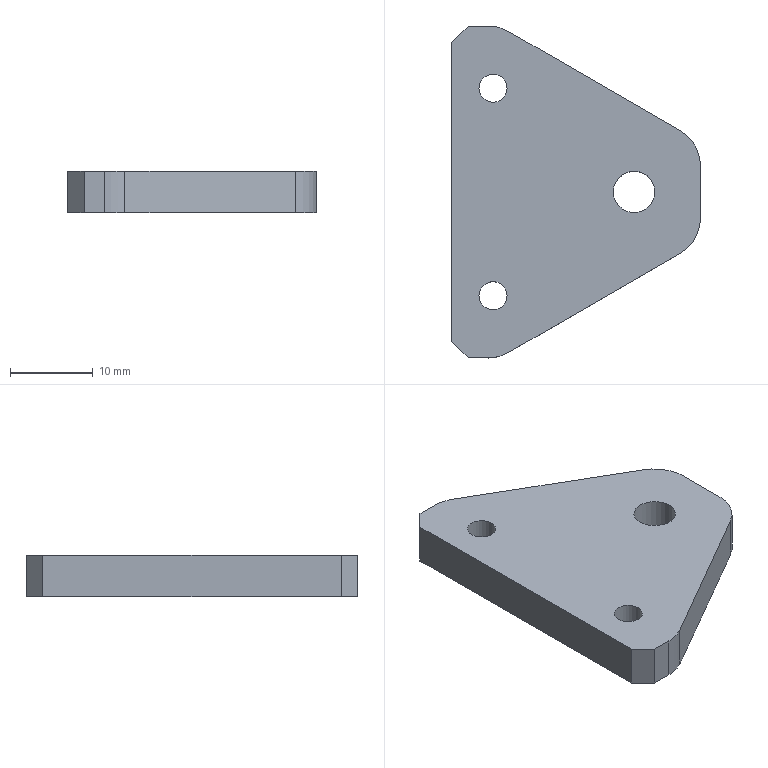Part | NX | 1 solid | 17 faces | box 30 x 40 x 5 mm | volume 4079 mm3 | plane 10 | cylinder 7 | commonest cylinder face diameters 10 x4 3.4 x2 5 x1
STEP:
#1=CARTESIAN_POINT('',(15.,-3.113,0.));
#2=VERTEX_POINT('',#1);
#3=CARTESIAN_POINT('',(15.,3.113,0.));
#4=VERTEX_POINT('',#3);
#5=CARTESIAN_POINT('',(15.,-20.,0.));
#6=DIRECTION('',(0.,1.,0.));
#7=VECTOR('',#6,1000.);
#8=LINE('',#5,#7);
#9=EDGE_CURVE('',#2,#4,#8,.T.);
#10=ORIENTED_EDGE('',*,*,#9,.F.);
#11=CARTESIAN_POINT('',(15.,-3.113,-5.));
#12=VERTEX_POINT('',#11);
#13=CARTESIAN_POINT('',(15.,-3.113,-5.));
#14=DIRECTION('',(0.,0.,1.));
#15=VECTOR('',#14,1000.);
#16=LINE('',#13,#15);
#17=EDGE_CURVE('',#2,#12,#16,.F.);
#18=ORIENTED_EDGE('',*,*,#17,.T.);
#19=CARTESIAN_POINT('',(15.,3.113,-5.));
#20=VERTEX_POINT('',#19);
#21=CARTESIAN_POINT('',(15.,-20.,-5.));
#22=DIRECTION('',(0.,1.,0.));
#23=VECTOR('',#22,1000.);
#24=LINE('',#21,#23);
#25=EDGE_CURVE('',#12,#20,#24,.T.);
#26=ORIENTED_EDGE('',*,*,#25,.T.);
#27=CARTESIAN_POINT('',(15.,3.113,-5.));
#28=DIRECTION('',(0.,0.,-1.));
#29=VECTOR('',#28,1000.);
#30=LINE('',#27,#29);
#31=EDGE_CURVE('',#20,#4,#30,.F.);
#32=ORIENTED_EDGE('',*,*,#31,.T.);
#33=EDGE_LOOP('',(#10,#18,#26,#32));
#34=FACE_BOUND('',#33,.T.);
#35=CARTESIAN_POINT('',(15.,-20.,-5.));
#36=DIRECTION('',(1.,0.,0.));
#37=DIRECTION('',(0.,0.,-1.));
#38=AXIS2_PLACEMENT_3D('',#35,#36,#37);
#39=PLANE('',#38);
#40=ADVANCED_FACE('',(#34),#39,.T.);
#41=CARTESIAN_POINT('',(-8.3,12.5,-5.));
#42=VERTEX_POINT('',#41);
#43=CARTESIAN_POINT('',(-10.,12.5,-5.));
#44=DIRECTION('',(0.,0.,1.));
#45=DIRECTION('',(1.,0.,0.));
#46=AXIS2_PLACEMENT_3D('',#43,#44,#45);
#47=CIRCLE('',#46,1.7);
#48=EDGE_CURVE('',#42,#42,#47,.T.);
#49=ORIENTED_EDGE('',*,*,#48,.T.);
#50=EDGE_LOOP('',(#49));
#51=FACE_BOUND('',#50,.T.);
#52=CARTESIAN_POINT('',(-8.3,-12.5,-5.));
#53=VERTEX_POINT('',#52);
#54=CARTESIAN_POINT('',(-10.,-12.5,-5.));
#55=DIRECTION('',(0.,0.,1.));
#56=DIRECTION('',(1.,0.,0.));
#57=AXIS2_PLACEMENT_3D('',#54,#55,#56);
#58=CIRCLE('',#57,1.7);
#59=EDGE_CURVE('',#53,#53,#58,.T.);
#60=ORIENTED_EDGE('',*,*,#59,.T.);
#61=EDGE_LOOP('',(#60));
#62=FACE_BOUND('',#61,.T.);
#63=CARTESIAN_POINT('',(9.5,0.,-5.));
#64=VERTEX_POINT('',#63);
#65=CARTESIAN_POINT('',(7.,0.,-5.));
#66=DIRECTION('',(0.,0.,1.));
#67=DIRECTION('',(1.,0.,0.));
#68=AXIS2_PLACEMENT_3D('',#65,#66,#67);
#69=CIRCLE('',#68,2.5);
#70=EDGE_CURVE('',#64,#64,#69,.T.);
#71=ORIENTED_EDGE('',*,*,#70,.T.);
#72=EDGE_LOOP('',(#71));
#73=FACE_BOUND('',#72,.T.);
#74=CARTESIAN_POINT('',(-13.,-20.,-5.));
#75=VERTEX_POINT('',#74);
#76=CARTESIAN_POINT('',(-10.588,-20.,-5.));
#77=VERTEX_POINT('',#76);
#78=CARTESIAN_POINT('',(-15.,-20.,-5.));
#79=DIRECTION('',(1.,0.,0.));
#80=VECTOR('',#79,1000.);
#81=LINE('',#78,#80);
#82=EDGE_CURVE('',#75,#77,#81,.T.);
#83=ORIENTED_EDGE('',*,*,#82,.F.);
#84=CARTESIAN_POINT('',(-15.,-18.,-5.));
#85=VERTEX_POINT('',#84);
#86=CARTESIAN_POINT('',(-16.5,-16.5,-5.));
#87=DIRECTION('',(0.7071,-0.7071,0.));
#88=VECTOR('',#87,1000.);
#89=LINE('',#86,#88);
#90=EDGE_CURVE('',#75,#85,#89,.F.);
#91=ORIENTED_EDGE('',*,*,#90,.T.);
#92=CARTESIAN_POINT('',(-15.,18.,-5.));
#93=VERTEX_POINT('',#92);
#94=CARTESIAN_POINT('',(-15.,-20.,-5.));
#95=DIRECTION('',(0.,-1.,0.));
#96=VECTOR('',#95,1000.);
#97=LINE('',#94,#96);
#98=EDGE_CURVE('',#93,#85,#97,.T.);
#99=ORIENTED_EDGE('',*,*,#98,.F.);
#100=CARTESIAN_POINT('',(-13.,20.,-5.));
#101=VERTEX_POINT('',#100);
#102=CARTESIAN_POINT('',(-16.5,16.5,-5.));
#103=DIRECTION('',(-0.7071,-0.7071,0.));
#104=VECTOR('',#103,1000.);
#105=LINE('',#102,#104);
#106=EDGE_CURVE('',#93,#101,#105,.F.);
#107=ORIENTED_EDGE('',*,*,#106,.T.);
#108=CARTESIAN_POINT('',(-10.588,20.,-5.));
#109=VERTEX_POINT('',#108);
#110=CARTESIAN_POINT('',(-15.,20.,-5.));
#111=DIRECTION('',(-1.,0.,0.));
#112=VECTOR('',#111,1000.);
#113=LINE('',#110,#112);
#114=EDGE_CURVE('',#109,#101,#113,.T.);
#115=ORIENTED_EDGE('',*,*,#114,.F.);
#116=CARTESIAN_POINT('',(-8.088,19.33,-5.));
#117=VERTEX_POINT('',#116);
#118=CARTESIAN_POINT('',(-10.588,15.,-5.));
#119=DIRECTION('',(0.,0.,-1.));
#120=DIRECTION('',(-1.,0.,0.));
#121=AXIS2_PLACEMENT_3D('',#118,#119,#120);
#122=CIRCLE('',#121,5.);
#123=EDGE_CURVE('',#109,#117,#122,.T.);
#124=ORIENTED_EDGE('',*,*,#123,.T.);
#125=CARTESIAN_POINT('',(12.5,7.443,-5.));
#126=VERTEX_POINT('',#125);
#127=CARTESIAN_POINT('',(-9.249,20.,-5.));
#128=DIRECTION('',(0.866,-0.5,0.));
#129=VECTOR('',#128,1000.);
#130=LINE('',#127,#129);
#131=EDGE_CURVE('',#117,#126,#130,.T.);
#132=ORIENTED_EDGE('',*,*,#131,.T.);
#133=CARTESIAN_POINT('',(10.,3.113,-5.));
#134=DIRECTION('',(0.,0.,-1.));
#135=DIRECTION('',(-1.,0.,0.));
#136=AXIS2_PLACEMENT_3D('',#133,#134,#135);
#137=CIRCLE('',#136,5.);
#138=EDGE_CURVE('',#126,#20,#137,.T.);
#139=ORIENTED_EDGE('',*,*,#138,.T.);
#140=ORIENTED_EDGE('',*,*,#25,.F.);
#141=CARTESIAN_POINT('',(12.5,-7.443,-5.));
#142=VERTEX_POINT('',#141);
#143=CARTESIAN_POINT('',(10.,-3.113,-5.));
#144=DIRECTION('',(0.,0.,-1.));
#145=DIRECTION('',(-1.,0.,0.));
#146=AXIS2_PLACEMENT_3D('',#143,#144,#145);
#147=CIRCLE('',#146,5.);
#148=EDGE_CURVE('',#12,#142,#147,.T.);
#149=ORIENTED_EDGE('',*,*,#148,.T.);
#150=CARTESIAN_POINT('',(-8.088,-19.33,-5.));
#151=VERTEX_POINT('',#150);
#152=CARTESIAN_POINT('',(-9.249,-20.,-5.));
#153=DIRECTION('',(0.866,0.5,0.));
#154=VECTOR('',#153,1000.);
#155=LINE('',#152,#154);
#156=EDGE_CURVE('',#151,#142,#155,.T.);
#157=ORIENTED_EDGE('',*,*,#156,.F.);
#158=CARTESIAN_POINT('',(-10.588,-15.,-5.));
#159=DIRECTION('',(0.,0.,-1.));
#160=DIRECTION('',(-1.,0.,0.));
#161=AXIS2_PLACEMENT_3D('',#158,#159,#160);
#162=CIRCLE('',#161,5.);
#163=EDGE_CURVE('',#151,#77,#162,.T.);
#164=ORIENTED_EDGE('',*,*,#163,.T.);
#165=EDGE_LOOP('',(#83,#91,#99,#107,#115,#124,#132,#139,#140,#149,#157,#164));
#166=FACE_BOUND('',#165,.T.);
#167=CARTESIAN_POINT('',(0.,0.,-5.));
#168=DIRECTION('',(0.,0.,-1.));
#169=DIRECTION('',(-1.,0.,0.));
#170=AXIS2_PLACEMENT_3D('',#167,#168,#169);
#171=PLANE('',#170);
#172=ADVANCED_FACE('',(#51,#62,#73,#166),#171,.T.);
#173=CARTESIAN_POINT('',(-8.3,12.5,0.));
#174=VERTEX_POINT('',#173);
#175=CARTESIAN_POINT('',(-10.,12.5,0.));
#176=DIRECTION('',(0.,0.,1.));
#177=DIRECTION('',(1.,0.,0.));
#178=AXIS2_PLACEMENT_3D('',#175,#176,#177);
#179=CIRCLE('',#178,1.7);
#180=EDGE_CURVE('',#174,#174,#179,.T.);
#181=ORIENTED_EDGE('',*,*,#180,.F.);
#182=EDGE_LOOP('',(#181));
#183=FACE_BOUND('',#182,.T.);
#184=CARTESIAN_POINT('',(-8.3,-12.5,0.));
#185=VERTEX_POINT('',#184);
#186=CARTESIAN_POINT('',(-10.,-12.5,0.));
#187=DIRECTION('',(0.,0.,1.));
#188=DIRECTION('',(1.,0.,0.));
#189=AXIS2_PLACEMENT_3D('',#186,#187,#188);
#190=CIRCLE('',#189,1.7);
#191=EDGE_CURVE('',#185,#185,#190,.T.);
#192=ORIENTED_EDGE('',*,*,#191,.F.);
#193=EDGE_LOOP('',(#192));
#194=FACE_BOUND('',#193,.T.);
#195=CARTESIAN_POINT('',(9.5,0.,0.));
#196=VERTEX_POINT('',#195);
#197=CARTESIAN_POINT('',(7.,0.,0.));
#198=DIRECTION('',(0.,0.,1.));
#199=DIRECTION('',(1.,0.,0.));
#200=AXIS2_PLACEMENT_3D('',#197,#198,#199);
#201=CIRCLE('',#200,2.5);
#202=EDGE_CURVE('',#196,#196,#201,.T.);
#203=ORIENTED_EDGE('',*,*,#202,.F.);
#204=EDGE_LOOP('',(#203));
#205=FACE_BOUND('',#204,.T.);
#206=CARTESIAN_POINT('',(-15.,18.,0.));
#207=VERTEX_POINT('',#206);
#208=CARTESIAN_POINT('',(-15.,-18.,0.));
#209=VERTEX_POINT('',#208);
#210=CARTESIAN_POINT('',(-15.,-20.,0.));
#211=DIRECTION('',(0.,-1.,0.));
#212=VECTOR('',#211,1000.);
#213=LINE('',#210,#212);
#214=EDGE_CURVE('',#207,#209,#213,.T.);
#215=ORIENTED_EDGE('',*,*,#214,.T.);
#216=CARTESIAN_POINT('',(-13.,-20.,0.));
#217=VERTEX_POINT('',#216);
#218=CARTESIAN_POINT('',(-15.,-18.,0.));
#219=DIRECTION('',(-0.7071,0.7071,0.));
#220=VECTOR('',#219,1000.);
#221=LINE('',#218,#220);
#222=EDGE_CURVE('',#209,#217,#221,.F.);
#223=ORIENTED_EDGE('',*,*,#222,.T.);
#224=CARTESIAN_POINT('',(-10.588,-20.,0.));
#225=VERTEX_POINT('',#224);
#226=CARTESIAN_POINT('',(-15.,-20.,0.));
#227=DIRECTION('',(1.,0.,0.));
#228=VECTOR('',#227,1000.);
#229=LINE('',#226,#228);
#230=EDGE_CURVE('',#217,#225,#229,.T.);
#231=ORIENTED_EDGE('',*,*,#230,.T.);
#232=CARTESIAN_POINT('',(-8.088,-19.33,0.));
#233=VERTEX_POINT('',#232);
#234=CARTESIAN_POINT('',(-10.588,-15.,0.));
#235=DIRECTION('',(0.,0.,-1.));
#236=DIRECTION('',(-1.,0.,0.));
#237=AXIS2_PLACEMENT_3D('',#234,#235,#236);
#238=CIRCLE('',#237,5.);
#239=EDGE_CURVE('',#225,#233,#238,.F.);
#240=ORIENTED_EDGE('',*,*,#239,.T.);
#241=CARTESIAN_POINT('',(12.5,-7.443,0.));
#242=VERTEX_POINT('',#241);
#243=CARTESIAN_POINT('',(-9.249,-20.,0.));
#244=DIRECTION('',(0.866,0.5,0.));
#245=VECTOR('',#244,1000.);
#246=LINE('',#243,#245);
#247=EDGE_CURVE('',#233,#242,#246,.T.);
#248=ORIENTED_EDGE('',*,*,#247,.T.);
#249=CARTESIAN_POINT('',(10.,-3.113,0.));
#250=DIRECTION('',(0.,0.,-1.));
#251=DIRECTION('',(-1.,0.,0.));
#252=AXIS2_PLACEMENT_3D('',#249,#250,#251);
#253=CIRCLE('',#252,5.);
#254=EDGE_CURVE('',#242,#2,#253,.F.);
#255=ORIENTED_EDGE('',*,*,#254,.T.);
#256=ORIENTED_EDGE('',*,*,#9,.T.);
#257=CARTESIAN_POINT('',(12.5,7.443,0.));
#258=VERTEX_POINT('',#257);
#259=CARTESIAN_POINT('',(10.,3.113,0.));
#260=DIRECTION('',(0.,0.,-1.));
#261=DIRECTION('',(-1.,0.,0.));
#262=AXIS2_PLACEMENT_3D('',#259,#260,#261);
#263=CIRCLE('',#262,5.);
#264=EDGE_CURVE('',#4,#258,#263,.F.);
#265=ORIENTED_EDGE('',*,*,#264,.T.);
#266=CARTESIAN_POINT('',(-8.088,19.33,0.));
#267=VERTEX_POINT('',#266);
#268=CARTESIAN_POINT('',(-9.249,20.,0.));
#269=DIRECTION('',(0.866,-0.5,0.));
#270=VECTOR('',#269,1000.);
#271=LINE('',#268,#270);
#272=EDGE_CURVE('',#267,#258,#271,.T.);
#273=ORIENTED_EDGE('',*,*,#272,.F.);
#274=CARTESIAN_POINT('',(-10.588,20.,0.));
#275=VERTEX_POINT('',#274);
#276=CARTESIAN_POINT('',(-10.588,15.,0.));
#277=DIRECTION('',(0.,0.,-1.));
#278=DIRECTION('',(-1.,0.,0.));
#279=AXIS2_PLACEMENT_3D('',#276,#277,#278);
#280=CIRCLE('',#279,5.);
#281=EDGE_CURVE('',#267,#275,#280,.F.);
#282=ORIENTED_EDGE('',*,*,#281,.T.);
#283=CARTESIAN_POINT('',(-13.,20.,0.));
#284=VERTEX_POINT('',#283);
#285=CARTESIAN_POINT('',(-15.,20.,0.));
#286=DIRECTION('',(-1.,0.,0.));
#287=VECTOR('',#286,1000.);
#288=LINE('',#285,#287);
#289=EDGE_CURVE('',#275,#284,#288,.T.);
#290=ORIENTED_EDGE('',*,*,#289,.T.);
#291=CARTESIAN_POINT('',(-13.,20.,0.));
#292=DIRECTION('',(0.7071,0.7071,0.));
#293=VECTOR('',#292,1000.);
#294=LINE('',#291,#293);
#295=EDGE_CURVE('',#284,#207,#294,.F.);
#296=ORIENTED_EDGE('',*,*,#295,.T.);
#297=EDGE_LOOP('',(#215,#223,#231,#240,#248,#255,#256,#265,#273,#282,#290,#296));
#298=FACE_BOUND('',#297,.T.);
#299=CARTESIAN_POINT('',(0.,0.,0.));
#300=DIRECTION('',(0.,0.,-1.));
#301=DIRECTION('',(-1.,0.,0.));
#302=AXIS2_PLACEMENT_3D('',#299,#300,#301);
#303=PLANE('',#302);
#304=ADVANCED_FACE('',(#183,#194,#205,#298),#303,.F.);
#305=ORIENTED_EDGE('',*,*,#230,.F.);
#306=CARTESIAN_POINT('',(-13.,-20.,-5.));
#307=DIRECTION('',(0.,0.,-1.));
#308=VECTOR('',#307,1000.);
#309=LINE('',#306,#308);
#310=EDGE_CURVE('',#217,#75,#309,.T.);
#311=ORIENTED_EDGE('',*,*,#310,.T.);
#312=ORIENTED_EDGE('',*,*,#82,.T.);
#313=CARTESIAN_POINT('',(-10.588,-20.,-5.));
#314=DIRECTION('',(0.,0.,1.));
#315=VECTOR('',#314,1000.);
#316=LINE('',#313,#315);
#317=EDGE_CURVE('',#77,#225,#316,.T.);
#318=ORIENTED_EDGE('',*,*,#317,.T.);
#319=EDGE_LOOP('',(#305,#311,#312,#318));
#320=FACE_BOUND('',#319,.T.);
#321=CARTESIAN_POINT('',(-15.,-20.,-5.));
#322=DIRECTION('',(0.,-1.,0.));
#323=DIRECTION('',(0.,0.,-1.));
#324=AXIS2_PLACEMENT_3D('',#321,#322,#323);
#325=PLANE('',#324);
#326=ADVANCED_FACE('',(#320),#325,.T.);
#327=ORIENTED_EDGE('',*,*,#114,.T.);
#328=CARTESIAN_POINT('',(-13.,20.,-5.));
#329=DIRECTION('',(0.,0.,1.));
#330=VECTOR('',#329,1000.);
#331=LINE('',#328,#330);
#332=EDGE_CURVE('',#101,#284,#331,.T.);
#333=ORIENTED_EDGE('',*,*,#332,.T.);
#334=ORIENTED_EDGE('',*,*,#289,.F.);
#335=CARTESIAN_POINT('',(-10.588,20.,-5.));
#336=DIRECTION('',(0.,0.,-1.));
#337=VECTOR('',#336,1000.);
#338=LINE('',#335,#337);
#339=EDGE_CURVE('',#275,#109,#338,.T.);
#340=ORIENTED_EDGE('',*,*,#339,.T.);
#341=EDGE_LOOP('',(#327,#333,#334,#340));
#342=FACE_BOUND('',#341,.T.);
#343=CARTESIAN_POINT('',(-15.,20.,-5.));
#344=DIRECTION('',(0.,1.,0.));
#345=DIRECTION('',(0.,0.,1.));
#346=AXIS2_PLACEMENT_3D('',#343,#344,#345);
#347=PLANE('',#346);
#348=ADVANCED_FACE('',(#342),#347,.T.);
#349=ORIENTED_EDGE('',*,*,#98,.T.);
#350=CARTESIAN_POINT('',(-15.,-18.,-5.));
#351=DIRECTION('',(0.,0.,1.));
#352=VECTOR('',#351,1000.);
#353=LINE('',#350,#352);
#354=EDGE_CURVE('',#85,#209,#353,.T.);
#355=ORIENTED_EDGE('',*,*,#354,.T.);
#356=ORIENTED_EDGE('',*,*,#214,.F.);
#357=CARTESIAN_POINT('',(-15.,18.,-5.));
#358=DIRECTION('',(0.,0.,-1.));
#359=VECTOR('',#358,1000.);
#360=LINE('',#357,#359);
#361=EDGE_CURVE('',#207,#93,#360,.T.);
#362=ORIENTED_EDGE('',*,*,#361,.T.);
#363=EDGE_LOOP('',(#349,#355,#356,#362));
#364=FACE_BOUND('',#363,.T.);
#365=CARTESIAN_POINT('',(-15.,-20.,-5.));
#366=DIRECTION('',(-1.,0.,0.));
#367=DIRECTION('',(0.,0.,1.));
#368=AXIS2_PLACEMENT_3D('',#365,#366,#367);
#369=PLANE('',#368);
#370=ADVANCED_FACE('',(#364),#369,.T.);
#371=ORIENTED_EDGE('',*,*,#131,.F.);
#372=CARTESIAN_POINT('',(-8.088,19.33,0.));
#373=DIRECTION('',(0.,0.,-1.));
#374=VECTOR('',#373,1000.);
#375=LINE('',#372,#374);
#376=EDGE_CURVE('',#117,#267,#375,.F.);
#377=ORIENTED_EDGE('',*,*,#376,.T.);
#378=ORIENTED_EDGE('',*,*,#272,.T.);
#379=CARTESIAN_POINT('',(12.5,7.443,0.));
#380=DIRECTION('',(0.,0.,-1.));
#381=VECTOR('',#380,1000.);
#382=LINE('',#379,#381);
#383=EDGE_CURVE('',#258,#126,#382,.T.);
#384=ORIENTED_EDGE('',*,*,#383,.T.);
#385=EDGE_LOOP('',(#371,#377,#378,#384));
#386=FACE_BOUND('',#385,.T.);
#387=CARTESIAN_POINT('',(-9.249,20.,0.));
#388=DIRECTION('',(0.5,0.866,0.));
#389=DIRECTION('',(0.866,-0.5,0.));
#390=AXIS2_PLACEMENT_3D('',#387,#388,#389);
#391=PLANE('',#390);
#392=ADVANCED_FACE('',(#386),#391,.T.);
#393=ORIENTED_EDGE('',*,*,#247,.F.);
#394=CARTESIAN_POINT('',(-8.088,-19.33,0.));
#395=DIRECTION('',(0.,0.,-1.));
#396=VECTOR('',#395,1000.);
#397=LINE('',#394,#396);
#398=EDGE_CURVE('',#233,#151,#397,.T.);
#399=ORIENTED_EDGE('',*,*,#398,.T.);
#400=ORIENTED_EDGE('',*,*,#156,.T.);
#401=CARTESIAN_POINT('',(12.5,-7.443,0.));
#402=DIRECTION('',(0.,0.,-1.));
#403=VECTOR('',#402,1000.);
#404=LINE('',#401,#403);
#405=EDGE_CURVE('',#142,#242,#404,.F.);
#406=ORIENTED_EDGE('',*,*,#405,.T.);
#407=EDGE_LOOP('',(#393,#399,#400,#406));
#408=FACE_BOUND('',#407,.T.);
#409=CARTESIAN_POINT('',(-9.249,-20.,0.));
#410=DIRECTION('',(-0.5,0.866,0.));
#411=DIRECTION('',(0.866,0.5,0.));
#412=AXIS2_PLACEMENT_3D('',#409,#410,#411);
#413=PLANE('',#412);
#414=ADVANCED_FACE('',(#408),#413,.F.);
#415=ORIENTED_EDGE('',*,*,#70,.F.);
#416=EDGE_LOOP('',(#415));
#417=FACE_BOUND('',#416,.T.);
#418=ORIENTED_EDGE('',*,*,#202,.T.);
#419=EDGE_LOOP('',(#418));
#420=FACE_BOUND('',#419,.T.);
#421=CARTESIAN_POINT('',(7.,0.,0.));
#422=DIRECTION('',(0.,0.,1.));
#423=DIRECTION('',(1.,0.,0.));
#424=AXIS2_PLACEMENT_3D('',#421,#422,#423);
#425=CYLINDRICAL_SURFACE('',#424,2.5);
#426=ADVANCED_FACE('',(#417,#420),#425,.F.);
#427=ORIENTED_EDGE('',*,*,#59,.F.);
#428=EDGE_LOOP('',(#427));
#429=FACE_BOUND('',#428,.T.);
#430=ORIENTED_EDGE('',*,*,#191,.T.);
#431=EDGE_LOOP('',(#430));
#432=FACE_BOUND('',#431,.T.);
#433=CARTESIAN_POINT('',(-10.,-12.5,0.));
#434=DIRECTION('',(0.,0.,1.));
#435=DIRECTION('',(1.,0.,0.));
#436=AXIS2_PLACEMENT_3D('',#433,#434,#435);
#437=CYLINDRICAL_SURFACE('',#436,1.7);
#438=ADVANCED_FACE('',(#429,#432),#437,.F.);
#439=ORIENTED_EDGE('',*,*,#48,.F.);
#440=EDGE_LOOP('',(#439));
#441=FACE_BOUND('',#440,.T.);
#442=ORIENTED_EDGE('',*,*,#180,.T.);
#443=EDGE_LOOP('',(#442));
#444=FACE_BOUND('',#443,.T.);
#445=CARTESIAN_POINT('',(-10.,12.5,0.));
#446=DIRECTION('',(0.,0.,1.));
#447=DIRECTION('',(1.,0.,0.));
#448=AXIS2_PLACEMENT_3D('',#445,#446,#447);
#449=CYLINDRICAL_SURFACE('',#448,1.7);
#450=ADVANCED_FACE('',(#441,#444),#449,.F.);
#451=ORIENTED_EDGE('',*,*,#239,.F.);
#452=ORIENTED_EDGE('',*,*,#317,.F.);
#453=ORIENTED_EDGE('',*,*,#163,.F.);
#454=ORIENTED_EDGE('',*,*,#398,.F.);
#455=EDGE_LOOP('',(#451,#452,#453,#454));
#456=FACE_BOUND('',#455,.T.);
#457=CARTESIAN_POINT('',(-10.588,-15.,0.));
#458=DIRECTION('',(0.,0.,1.));
#459=DIRECTION('',(1.,0.,0.));
#460=AXIS2_PLACEMENT_3D('',#457,#458,#459);
#461=CYLINDRICAL_SURFACE('',#460,5.);
#462=ADVANCED_FACE('',(#456),#461,.T.);
#463=ORIENTED_EDGE('',*,*,#281,.F.);
#464=ORIENTED_EDGE('',*,*,#376,.F.);
#465=ORIENTED_EDGE('',*,*,#123,.F.);
#466=ORIENTED_EDGE('',*,*,#339,.F.);
#467=EDGE_LOOP('',(#463,#464,#465,#466));
#468=FACE_BOUND('',#467,.T.);
#469=CARTESIAN_POINT('',(-10.588,15.,-5.));
#470=DIRECTION('',(0.,0.,-1.));
#471=DIRECTION('',(-1.,0.,0.));
#472=AXIS2_PLACEMENT_3D('',#469,#470,#471);
#473=CYLINDRICAL_SURFACE('',#472,5.);
#474=ADVANCED_FACE('',(#468),#473,.T.);
#475=ORIENTED_EDGE('',*,*,#254,.F.);
#476=ORIENTED_EDGE('',*,*,#405,.F.);
#477=ORIENTED_EDGE('',*,*,#148,.F.);
#478=ORIENTED_EDGE('',*,*,#17,.F.);
#479=EDGE_LOOP('',(#475,#476,#477,#478));
#480=FACE_BOUND('',#479,.T.);
#481=CARTESIAN_POINT('',(10.,-3.113,-5.));
#482=DIRECTION('',(0.,0.,1.));
#483=DIRECTION('',(1.,0.,0.));
#484=AXIS2_PLACEMENT_3D('',#481,#482,#483);
#485=CYLINDRICAL_SURFACE('',#484,5.);
#486=ADVANCED_FACE('',(#480),#485,.T.);
#487=ORIENTED_EDGE('',*,*,#264,.F.);
#488=ORIENTED_EDGE('',*,*,#31,.F.);
#489=ORIENTED_EDGE('',*,*,#138,.F.);
#490=ORIENTED_EDGE('',*,*,#383,.F.);
#491=EDGE_LOOP('',(#487,#488,#489,#490));
#492=FACE_BOUND('',#491,.T.);
#493=CARTESIAN_POINT('',(10.,3.113,0.));
#494=DIRECTION('',(0.,0.,-1.));
#495=DIRECTION('',(-1.,0.,0.));
#496=AXIS2_PLACEMENT_3D('',#493,#494,#495);
#497=CYLINDRICAL_SURFACE('',#496,5.);
#498=ADVANCED_FACE('',(#492),#497,.T.);
#499=ORIENTED_EDGE('',*,*,#90,.F.);
#500=ORIENTED_EDGE('',*,*,#310,.F.);
#501=ORIENTED_EDGE('',*,*,#222,.F.);
#502=ORIENTED_EDGE('',*,*,#354,.F.);
#503=EDGE_LOOP('',(#499,#500,#501,#502));
#504=FACE_BOUND('',#503,.T.);
#505=CARTESIAN_POINT('',(-15.,-18.,-5.));
#506=DIRECTION('',(0.7071,0.7071,0.));
#507=DIRECTION('',(0.,0.,1.));
#508=AXIS2_PLACEMENT_3D('',#505,#506,#507);
#509=PLANE('',#508);
#510=ADVANCED_FACE('',(#504),#509,.F.);
#511=ORIENTED_EDGE('',*,*,#106,.F.);
#512=ORIENTED_EDGE('',*,*,#361,.F.);
#513=ORIENTED_EDGE('',*,*,#295,.F.);
#514=ORIENTED_EDGE('',*,*,#332,.F.);
#515=EDGE_LOOP('',(#511,#512,#513,#514));
#516=FACE_BOUND('',#515,.T.);
#517=CARTESIAN_POINT('',(-13.,20.,-5.));
#518=DIRECTION('',(0.7071,-0.7071,0.));
#519=DIRECTION('',(0.,0.,1.));
#520=AXIS2_PLACEMENT_3D('',#517,#518,#519);
#521=PLANE('',#520);
#522=ADVANCED_FACE('',(#516),#521,.F.);
#523=CLOSED_SHELL('',(#40,#172,#304,#326,#348,#370,#392,#414,#426,#438,#450,#462,#474,#486,#498,#510,#522));
#524=MANIFOLD_SOLID_BREP('',#523);
#525=(LENGTH_UNIT()NAMED_UNIT(*)SI_UNIT(.MILLI.,.METRE.));
#526=UNCERTAINTY_MEASURE_WITH_UNIT(LENGTH_MEASURE(0.00001),#525,'','');
#527=(NAMED_UNIT(*)PLANE_ANGLE_UNIT()SI_UNIT($,.RADIAN.));
#528=(NAMED_UNIT(*)SI_UNIT($,.STERADIAN.)SOLID_ANGLE_UNIT());
#529=(GEOMETRIC_REPRESENTATION_CONTEXT(3)GLOBAL_UNCERTAINTY_ASSIGNED_CONTEXT((#526))GLOBAL_UNIT_ASSIGNED_CONTEXT((#525,#527,#528))REPRESENTATION_CONTEXT('',''));
#530=ADVANCED_BREP_SHAPE_REPRESENTATION('',(#524),#529);